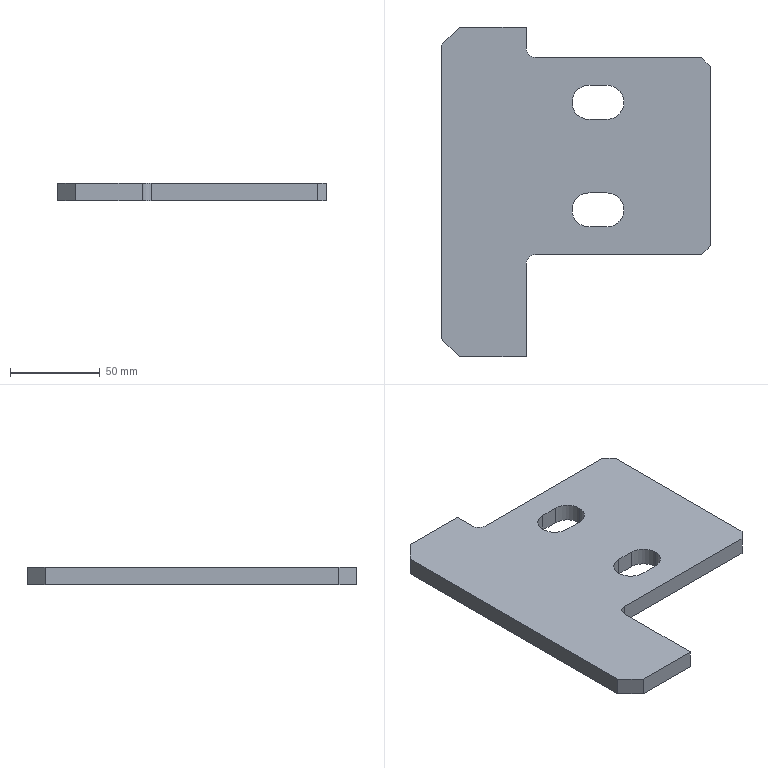Part | STEP file | Rib plate 200-16-1 | 1 solid | 26 faces | box 150 x 184 x 10 mm | volume 189352 mm3 | plane 18 | cylinder 8 | commonest cylinder face diameters 19 x6 10 x2